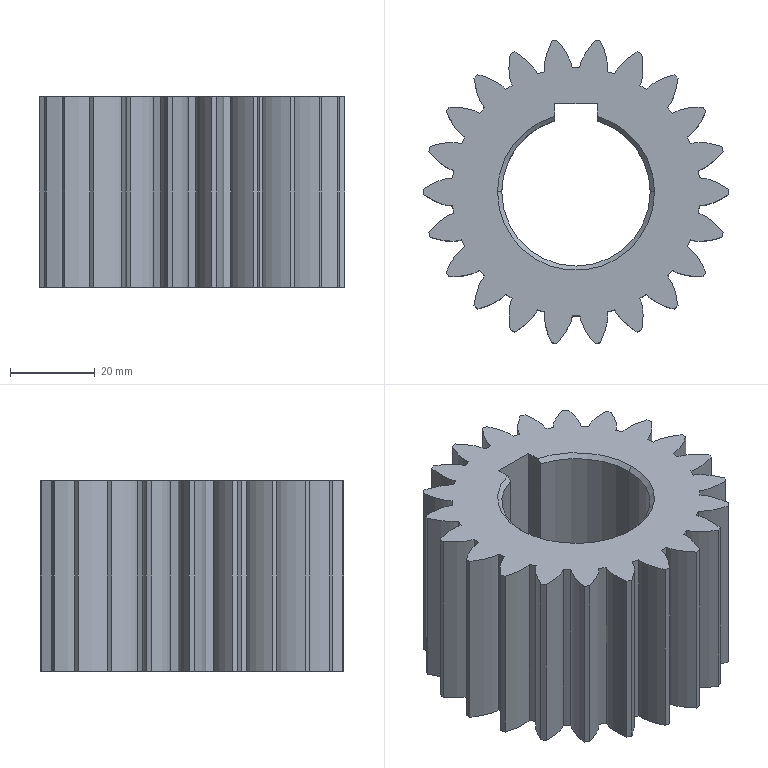Part | SolidWorks | features Chamfer 1, ICE 1, MBimport 1 | 1 solid | 102 faces | box 71.989 x 71.433 x 45 mm | volume 107206 mm3 | plane 49 | spline 44 | cone 6 | cylinder 3 | commonest cylinder face diameters 35 x3